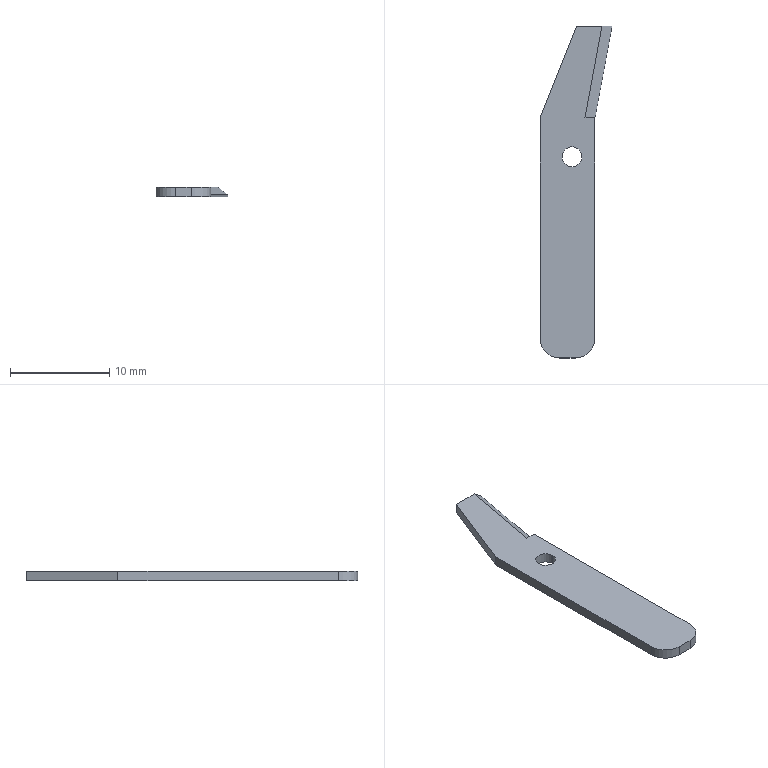Part | SolidWorks | features BaseBody 1, ICE 1 | 1 solid | 14 faces | box 7.242 x 33.391 x 1 mm | volume 166.861 mm3 | plane 10 | cylinder 4 | commonest cylinder face diameters 2 x2 4 x2
STEP:
#1=CARTESIAN_POINT('',(-123.21,229.702,181.));
#2=VERTEX_POINT('',#1);
#3=CARTESIAN_POINT('',(-121.21,229.702,181.));
#4=VERTEX_POINT('',#3);
#5=CARTESIAN_POINT('',(-122.21,229.702,181.));
#6=DIRECTION('',(0.,0.,1.));
#7=DIRECTION('',(0.,-1.,0.));
#8=AXIS2_PLACEMENT_3D('',#5,#6,#7);
#9=CIRCLE('',#8,1.);
#10=EDGE_CURVE('',#2,#4,#9,.T.);
#11=ORIENTED_EDGE('',*,*,#10,.T.);
#12=CARTESIAN_POINT('',(-121.21,229.702,180.));
#13=VERTEX_POINT('',#12);
#14=CARTESIAN_POINT('',(-121.21,229.702,181.));
#15=DIRECTION('',(0.,0.,-1.));
#16=VECTOR('',#15,1000.);
#17=LINE('',#14,#16);
#18=EDGE_CURVE('',#4,#13,#17,.T.);
#19=ORIENTED_EDGE('',*,*,#18,.T.);
#20=CARTESIAN_POINT('',(-123.21,229.702,180.));
#21=VERTEX_POINT('',#20);
#22=CARTESIAN_POINT('',(-122.21,229.702,180.));
#23=DIRECTION('',(0.,0.,1.));
#24=DIRECTION('',(0.,-1.,0.));
#25=AXIS2_PLACEMENT_3D('',#22,#23,#24);
#26=CIRCLE('',#25,1.);
#27=EDGE_CURVE('',#21,#13,#26,.T.);
#28=ORIENTED_EDGE('',*,*,#27,.F.);
#29=CARTESIAN_POINT('',(-123.21,229.702,181.));
#30=DIRECTION('',(0.,0.,-1.));
#31=VECTOR('',#30,1000.);
#32=LINE('',#29,#31);
#33=EDGE_CURVE('',#2,#21,#32,.T.);
#34=ORIENTED_EDGE('',*,*,#33,.F.);
#35=EDGE_LOOP('',(#11,#19,#28,#34));
#36=FACE_OUTER_BOUND('',#35,.T.);
#37=CARTESIAN_POINT('',(-122.21,229.702,181.));
#38=DIRECTION('',(0.,0.,-1.));
#39=DIRECTION('',(-1.,0.,0.));
#40=AXIS2_PLACEMENT_3D('',#37,#38,#39);
#41=CYLINDRICAL_SURFACE('',#40,1.);
#42=ADVANCED_FACE('',(#36),#41,.F.);
#43=CARTESIAN_POINT('',(-125.427,233.602,180.));
#44=VERTEX_POINT('',#43);
#45=CARTESIAN_POINT('',(-125.427,211.461,180.));
#46=VERTEX_POINT('',#45);
#47=CARTESIAN_POINT('',(-125.427,233.602,180.));
#48=DIRECTION('',(0.,-1.,0.));
#49=VECTOR('',#48,1000.);
#50=LINE('',#47,#49);
#51=EDGE_CURVE('',#44,#46,#50,.T.);
#52=ORIENTED_EDGE('',*,*,#51,.T.);
#53=CARTESIAN_POINT('',(-125.427,211.461,181.));
#54=VERTEX_POINT('',#53);
#55=CARTESIAN_POINT('',(-125.427,211.461,180.));
#56=DIRECTION('',(0.,0.,1.));
#57=VECTOR('',#56,1000.);
#58=LINE('',#55,#57);
#59=EDGE_CURVE('',#46,#54,#58,.T.);
#60=ORIENTED_EDGE('',*,*,#59,.T.);
#61=CARTESIAN_POINT('',(-125.427,233.602,181.));
#62=VERTEX_POINT('',#61);
#63=CARTESIAN_POINT('',(-125.427,233.602,181.));
#64=DIRECTION('',(0.,-1.,0.));
#65=VECTOR('',#64,1000.);
#66=LINE('',#63,#65);
#67=EDGE_CURVE('',#62,#54,#66,.T.);
#68=ORIENTED_EDGE('',*,*,#67,.F.);
#69=CARTESIAN_POINT('',(-125.427,233.602,181.));
#70=DIRECTION('',(0.,0.,-1.));
#71=VECTOR('',#70,1000.);
#72=LINE('',#69,#71);
#73=EDGE_CURVE('',#62,#44,#72,.T.);
#74=ORIENTED_EDGE('',*,*,#73,.T.);
#75=EDGE_LOOP('',(#52,#60,#68,#74));
#76=FACE_OUTER_BOUND('',#75,.T.);
#77=CARTESIAN_POINT('',(-125.427,233.602,181.));
#78=DIRECTION('',(1.,0.,0.));
#79=DIRECTION('',(0.,0.,-1.));
#80=AXIS2_PLACEMENT_3D('',#77,#78,#79);
#81=PLANE('',#80);
#82=ADVANCED_FACE('',(#76),#81,.F.);
#83=CARTESIAN_POINT('',(-119.902,233.602,180.2));
#84=VERTEX_POINT('',#83);
#85=CARTESIAN_POINT('',(-119.902,233.602,181.));
#86=VERTEX_POINT('',#85);
#87=CARTESIAN_POINT('',(-119.902,233.602,180.));
#88=DIRECTION('',(0.,0.,1.));
#89=VECTOR('',#88,1000.);
#90=LINE('',#87,#89);
#91=EDGE_CURVE('',#84,#86,#90,.T.);
#92=ORIENTED_EDGE('',*,*,#91,.T.);
#93=CARTESIAN_POINT('',(-119.902,211.461,181.));
#94=VERTEX_POINT('',#93);
#95=CARTESIAN_POINT('',(-119.902,220.3,181.));
#96=DIRECTION('',(0.,1.,0.));
#97=VECTOR('',#96,1000.);
#98=LINE('',#95,#97);
#99=EDGE_CURVE('',#94,#86,#98,.T.);
#100=ORIENTED_EDGE('',*,*,#99,.F.);
#101=CARTESIAN_POINT('',(-119.902,211.461,180.));
#102=VERTEX_POINT('',#101);
#103=CARTESIAN_POINT('',(-119.902,211.461,180.));
#104=DIRECTION('',(0.,0.,1.));
#105=VECTOR('',#104,1000.);
#106=LINE('',#103,#105);
#107=EDGE_CURVE('',#102,#94,#106,.T.);
#108=ORIENTED_EDGE('',*,*,#107,.F.);
#109=CARTESIAN_POINT('',(-119.902,233.602,180.));
#110=VERTEX_POINT('',#109);
#111=CARTESIAN_POINT('',(-119.902,220.3,180.));
#112=DIRECTION('',(0.,1.,0.));
#113=VECTOR('',#112,1000.);
#114=LINE('',#111,#113);
#115=EDGE_CURVE('',#102,#110,#114,.T.);
#116=ORIENTED_EDGE('',*,*,#115,.T.);
#117=CARTESIAN_POINT('',(-119.902,233.602,181.));
#118=DIRECTION('',(0.,0.,-1.));
#119=VECTOR('',#118,1000.);
#120=LINE('',#117,#119);
#121=EDGE_CURVE('',#84,#110,#120,.T.);
#122=ORIENTED_EDGE('',*,*,#121,.F.);
#123=EDGE_LOOP('',(#92,#100,#108,#116,#122));
#124=FACE_OUTER_BOUND('',#123,.T.);
#125=CARTESIAN_POINT('',(-119.902,220.3,181.));
#126=DIRECTION('',(-1.,0.,0.));
#127=DIRECTION('',(0.,0.,1.));
#128=AXIS2_PLACEMENT_3D('',#125,#126,#127);
#129=PLANE('',#128);
#130=ADVANCED_FACE('',(#124),#129,.F.);
#131=CARTESIAN_POINT('',(-118.186,242.853,180.2));
#132=VERTEX_POINT('',#131);
#133=CARTESIAN_POINT('',(-118.186,242.853,180.));
#134=VERTEX_POINT('',#133);
#135=CARTESIAN_POINT('',(-118.186,242.853,181.));
#136=DIRECTION('',(0.,0.,-1.));
#137=VECTOR('',#136,1000.);
#138=LINE('',#135,#137);
#139=EDGE_CURVE('',#132,#134,#138,.T.);
#140=ORIENTED_EDGE('',*,*,#139,.F.);
#141=CARTESIAN_POINT('',(-119.902,233.602,180.2));
#142=DIRECTION('',(-0.1825,-0.9832,0.));
#143=VECTOR('',#142,1000.);
#144=LINE('',#141,#143);
#145=EDGE_CURVE('',#132,#84,#144,.T.);
#146=ORIENTED_EDGE('',*,*,#145,.T.);
#147=ORIENTED_EDGE('',*,*,#121,.T.);
#148=CARTESIAN_POINT('',(-119.902,233.602,180.));
#149=DIRECTION('',(0.1825,0.9832,0.));
#150=VECTOR('',#149,1000.);
#151=LINE('',#148,#150);
#152=EDGE_CURVE('',#110,#134,#151,.T.);
#153=ORIENTED_EDGE('',*,*,#152,.T.);
#154=EDGE_LOOP('',(#140,#146,#147,#153));
#155=FACE_OUTER_BOUND('',#154,.T.);
#156=CARTESIAN_POINT('',(-119.902,233.602,181.));
#157=DIRECTION('',(-0.9832,0.1825,0.));
#158=DIRECTION('',(-0.1825,-0.9832,0.));
#159=AXIS2_PLACEMENT_3D('',#156,#157,#158);
#160=PLANE('',#159);
#161=ADVANCED_FACE('',(#155),#160,.F.);
#162=CARTESIAN_POINT('',(-119.203,242.853,181.));
#163=VERTEX_POINT('',#162);
#164=CARTESIAN_POINT('',(-121.763,242.853,181.));
#165=VERTEX_POINT('',#164);
#166=CARTESIAN_POINT('',(-118.186,242.853,181.));
#167=DIRECTION('',(-1.,0.,0.));
#168=VECTOR('',#167,1000.);
#169=LINE('',#166,#168);
#170=EDGE_CURVE('',#163,#165,#169,.T.);
#171=ORIENTED_EDGE('',*,*,#170,.F.);
#172=CARTESIAN_POINT('',(-120.722,242.853,182.195));
#173=DIRECTION('',(0.786,0.,-0.6182));
#174=VECTOR('',#173,1000.);
#175=LINE('',#172,#174);
#176=EDGE_CURVE('',#163,#132,#175,.T.);
#177=ORIENTED_EDGE('',*,*,#176,.T.);
#178=ORIENTED_EDGE('',*,*,#139,.T.);
#179=CARTESIAN_POINT('',(-121.763,242.853,180.));
#180=VERTEX_POINT('',#179);
#181=CARTESIAN_POINT('',(-118.186,242.853,180.));
#182=DIRECTION('',(-1.,0.,0.));
#183=VECTOR('',#182,1000.);
#184=LINE('',#181,#183);
#185=EDGE_CURVE('',#134,#180,#184,.T.);
#186=ORIENTED_EDGE('',*,*,#185,.T.);
#187=CARTESIAN_POINT('',(-121.763,242.853,181.));
#188=DIRECTION('',(0.,0.,-1.));
#189=VECTOR('',#188,1000.);
#190=LINE('',#187,#189);
#191=EDGE_CURVE('',#165,#180,#190,.T.);
#192=ORIENTED_EDGE('',*,*,#191,.F.);
#193=EDGE_LOOP('',(#171,#177,#178,#186,#192));
#194=FACE_OUTER_BOUND('',#193,.T.);
#195=CARTESIAN_POINT('',(-118.186,242.853,181.));
#196=DIRECTION('',(0.,-1.,0.));
#197=DIRECTION('',(0.,0.,-1.));
#198=AXIS2_PLACEMENT_3D('',#195,#196,#197);
#199=PLANE('',#198);
#200=ADVANCED_FACE('',(#194),#199,.F.);
#201=CARTESIAN_POINT('',(-121.763,242.853,180.));
#202=DIRECTION('',(-0.3683,-0.9297,0.));
#203=VECTOR('',#202,1000.);
#204=LINE('',#201,#203);
#205=EDGE_CURVE('',#180,#44,#204,.T.);
#206=ORIENTED_EDGE('',*,*,#205,.T.);
#207=ORIENTED_EDGE('',*,*,#73,.F.);
#208=CARTESIAN_POINT('',(-121.763,242.853,181.));
#209=DIRECTION('',(-0.3683,-0.9297,0.));
#210=VECTOR('',#209,1000.);
#211=LINE('',#208,#210);
#212=EDGE_CURVE('',#165,#62,#211,.T.);
#213=ORIENTED_EDGE('',*,*,#212,.F.);
#214=ORIENTED_EDGE('',*,*,#191,.T.);
#215=EDGE_LOOP('',(#206,#207,#213,#214));
#216=FACE_OUTER_BOUND('',#215,.T.);
#217=CARTESIAN_POINT('',(-121.763,242.853,181.));
#218=DIRECTION('',(0.9297,-0.3683,0.));
#219=DIRECTION('',(0.3683,0.9297,0.));
#220=AXIS2_PLACEMENT_3D('',#217,#218,#219);
#221=PLANE('',#220);
#222=ADVANCED_FACE('',(#216),#221,.F.);
#223=ORIENTED_EDGE('',*,*,#18,.F.);
#224=CARTESIAN_POINT('',(-122.21,229.702,181.));
#225=DIRECTION('',(0.,0.,1.));
#226=DIRECTION('',(0.,-1.,0.));
#227=AXIS2_PLACEMENT_3D('',#224,#225,#226);
#228=CIRCLE('',#227,1.);
#229=EDGE_CURVE('',#4,#2,#228,.T.);
#230=ORIENTED_EDGE('',*,*,#229,.T.);
#231=ORIENTED_EDGE('',*,*,#33,.T.);
#232=CARTESIAN_POINT('',(-122.21,229.702,180.));
#233=DIRECTION('',(0.,0.,1.));
#234=DIRECTION('',(0.,-1.,0.));
#235=AXIS2_PLACEMENT_3D('',#232,#233,#234);
#236=CIRCLE('',#235,1.);
#237=EDGE_CURVE('',#13,#21,#236,.T.);
#238=ORIENTED_EDGE('',*,*,#237,.F.);
#239=EDGE_LOOP('',(#223,#230,#231,#238));
#240=FACE_OUTER_BOUND('',#239,.T.);
#241=CARTESIAN_POINT('',(-122.21,229.702,181.));
#242=DIRECTION('',(0.,0.,-1.));
#243=DIRECTION('',(-1.,0.,0.));
#244=AXIS2_PLACEMENT_3D('',#241,#242,#243);
#245=CYLINDRICAL_SURFACE('',#244,1.);
#246=ADVANCED_FACE('',(#240),#245,.F.);
#247=ORIENTED_EDGE('',*,*,#67,.T.);
#248=CARTESIAN_POINT('',(-123.427,209.461,181.));
#249=VERTEX_POINT('',#248);
#250=CARTESIAN_POINT('',(-123.427,211.461,181.));
#251=DIRECTION('',(0.,0.,1.));
#252=DIRECTION('',(1.,0.,0.));
#253=AXIS2_PLACEMENT_3D('',#250,#251,#252);
#254=CIRCLE('',#253,2.);
#255=EDGE_CURVE('',#54,#249,#254,.T.);
#256=ORIENTED_EDGE('',*,*,#255,.T.);
#257=CARTESIAN_POINT('',(-121.902,209.461,181.));
#258=VERTEX_POINT('',#257);
#259=CARTESIAN_POINT('',(-123.427,209.461,181.));
#260=DIRECTION('',(1.,0.,0.));
#261=VECTOR('',#260,1000.);
#262=LINE('',#259,#261);
#263=EDGE_CURVE('',#249,#258,#262,.T.);
#264=ORIENTED_EDGE('',*,*,#263,.T.);
#265=CARTESIAN_POINT('',(-121.902,211.461,181.));
#266=DIRECTION('',(0.,0.,1.));
#267=DIRECTION('',(-1.,0.,0.));
#268=AXIS2_PLACEMENT_3D('',#265,#266,#267);
#269=CIRCLE('',#268,2.);
#270=EDGE_CURVE('',#258,#94,#269,.T.);
#271=ORIENTED_EDGE('',*,*,#270,.T.);
#272=ORIENTED_EDGE('',*,*,#99,.T.);
#273=CARTESIAN_POINT('',(-120.902,233.694,181.));
#274=VERTEX_POINT('',#273);
#275=CARTESIAN_POINT('',(-119.902,233.602,181.));
#276=DIRECTION('',(-0.9958,0.09162,0.));
#277=VECTOR('',#276,1000.);
#278=LINE('',#275,#277);
#279=EDGE_CURVE('',#86,#274,#278,.T.);
#280=ORIENTED_EDGE('',*,*,#279,.T.);
#281=CARTESIAN_POINT('',(-119.169,243.035,181.));
#282=DIRECTION('',(0.1825,0.9832,0.));
#283=VECTOR('',#282,1000.);
#284=LINE('',#281,#283);
#285=EDGE_CURVE('',#274,#163,#284,.T.);
#286=ORIENTED_EDGE('',*,*,#285,.T.);
#287=ORIENTED_EDGE('',*,*,#170,.T.);
#288=ORIENTED_EDGE('',*,*,#212,.T.);
#289=EDGE_LOOP('',(#247,#256,#264,#271,#272,#280,#286,#287,#288));
#290=FACE_OUTER_BOUND('',#289,.T.);
#291=ORIENTED_EDGE('',*,*,#10,.F.);
#292=ORIENTED_EDGE('',*,*,#229,.F.);
#293=EDGE_LOOP('',(#291,#292));
#294=FACE_BOUND('',#293,.T.);
#295=CARTESIAN_POINT('',(-122.21,229.702,181.));
#296=DIRECTION('',(0.,0.,1.));
#297=DIRECTION('',(1.,0.,0.));
#298=AXIS2_PLACEMENT_3D('',#295,#296,#297);
#299=PLANE('',#298);
#300=ADVANCED_FACE('',(#290,#294),#299,.T.);
#301=ORIENTED_EDGE('',*,*,#152,.F.);
#302=ORIENTED_EDGE('',*,*,#115,.F.);
#303=CARTESIAN_POINT('',(-121.902,209.461,180.));
#304=VERTEX_POINT('',#303);
#305=CARTESIAN_POINT('',(-121.902,211.461,180.));
#306=DIRECTION('',(0.,0.,1.));
#307=DIRECTION('',(-1.,0.,0.));
#308=AXIS2_PLACEMENT_3D('',#305,#306,#307);
#309=CIRCLE('',#308,2.);
#310=EDGE_CURVE('',#304,#102,#309,.T.);
#311=ORIENTED_EDGE('',*,*,#310,.F.);
#312=CARTESIAN_POINT('',(-123.427,209.461,180.));
#313=VERTEX_POINT('',#312);
#314=CARTESIAN_POINT('',(-123.427,209.461,180.));
#315=DIRECTION('',(1.,0.,0.));
#316=VECTOR('',#315,1000.);
#317=LINE('',#314,#316);
#318=EDGE_CURVE('',#313,#304,#317,.T.);
#319=ORIENTED_EDGE('',*,*,#318,.F.);
#320=CARTESIAN_POINT('',(-123.427,211.461,180.));
#321=DIRECTION('',(0.,0.,1.));
#322=DIRECTION('',(1.,0.,0.));
#323=AXIS2_PLACEMENT_3D('',#320,#321,#322);
#324=CIRCLE('',#323,2.);
#325=EDGE_CURVE('',#46,#313,#324,.T.);
#326=ORIENTED_EDGE('',*,*,#325,.F.);
#327=ORIENTED_EDGE('',*,*,#51,.F.);
#328=ORIENTED_EDGE('',*,*,#205,.F.);
#329=ORIENTED_EDGE('',*,*,#185,.F.);
#330=EDGE_LOOP('',(#301,#302,#311,#319,#326,#327,#328,#329));
#331=FACE_OUTER_BOUND('',#330,.T.);
#332=ORIENTED_EDGE('',*,*,#27,.T.);
#333=ORIENTED_EDGE('',*,*,#237,.T.);
#334=EDGE_LOOP('',(#332,#333));
#335=FACE_BOUND('',#334,.T.);
#336=CARTESIAN_POINT('',(-122.21,229.702,180.));
#337=DIRECTION('',(0.,0.,1.));
#338=DIRECTION('',(1.,0.,0.));
#339=AXIS2_PLACEMENT_3D('',#336,#337,#338);
#340=PLANE('',#339);
#341=ADVANCED_FACE('',(#331,#335),#340,.F.);
#342=ORIENTED_EDGE('',*,*,#176,.F.);
#343=ORIENTED_EDGE('',*,*,#285,.F.);
#344=CARTESIAN_POINT('',(-120.68,233.673,180.822));
#345=DIRECTION('',(-0.7789,0.07166,0.6231));
#346=VECTOR('',#345,1000.);
#347=LINE('',#344,#346);
#348=EDGE_CURVE('',#84,#274,#347,.T.);
#349=ORIENTED_EDGE('',*,*,#348,.F.);
#350=ORIENTED_EDGE('',*,*,#145,.F.);
#351=EDGE_LOOP('',(#342,#343,#349,#350));
#352=FACE_OUTER_BOUND('',#351,.T.);
#353=CARTESIAN_POINT('',(-121.662,229.6,181.));
#354=DIRECTION('',(0.6142,-0.114,0.7809));
#355=DIRECTION('',(-0.1825,-0.9832,0.));
#356=AXIS2_PLACEMENT_3D('',#353,#354,#355);
#357=PLANE('',#356);
#358=ADVANCED_FACE('',(#352),#357,.T.);
#359=ORIENTED_EDGE('',*,*,#91,.F.);
#360=ORIENTED_EDGE('',*,*,#348,.T.);
#361=ORIENTED_EDGE('',*,*,#279,.F.);
#362=EDGE_LOOP('',(#359,#360,#361));
#363=FACE_OUTER_BOUND('',#362,.T.);
#364=CARTESIAN_POINT('',(-119.902,233.602,180.));
#365=DIRECTION('',(0.09162,0.9958,0.));
#366=DIRECTION('',(-0.9958,0.09162,0.));
#367=AXIS2_PLACEMENT_3D('',#364,#365,#366);
#368=PLANE('',#367);
#369=ADVANCED_FACE('',(#363),#368,.T.);
#370=ORIENTED_EDGE('',*,*,#270,.F.);
#371=CARTESIAN_POINT('',(-121.902,209.461,180.));
#372=DIRECTION('',(0.,0.,1.));
#373=VECTOR('',#372,1000.);
#374=LINE('',#371,#373);
#375=EDGE_CURVE('',#304,#258,#374,.T.);
#376=ORIENTED_EDGE('',*,*,#375,.F.);
#377=ORIENTED_EDGE('',*,*,#310,.T.);
#378=ORIENTED_EDGE('',*,*,#107,.T.);
#379=EDGE_LOOP('',(#370,#376,#377,#378));
#380=FACE_OUTER_BOUND('',#379,.T.);
#381=CARTESIAN_POINT('',(-121.902,211.461,180.));
#382=DIRECTION('',(0.,0.,1.));
#383=DIRECTION('',(1.,0.,0.));
#384=AXIS2_PLACEMENT_3D('',#381,#382,#383);
#385=CYLINDRICAL_SURFACE('',#384,2.);
#386=ADVANCED_FACE('',(#380),#385,.T.);
#387=ORIENTED_EDGE('',*,*,#263,.F.);
#388=CARTESIAN_POINT('',(-123.427,209.461,180.));
#389=DIRECTION('',(0.,0.,1.));
#390=VECTOR('',#389,1000.);
#391=LINE('',#388,#390);
#392=EDGE_CURVE('',#313,#249,#391,.T.);
#393=ORIENTED_EDGE('',*,*,#392,.F.);
#394=ORIENTED_EDGE('',*,*,#318,.T.);
#395=ORIENTED_EDGE('',*,*,#375,.T.);
#396=EDGE_LOOP('',(#387,#393,#394,#395));
#397=FACE_OUTER_BOUND('',#396,.T.);
#398=CARTESIAN_POINT('',(-123.427,209.461,180.));
#399=DIRECTION('',(0.,-1.,0.));
#400=DIRECTION('',(0.,0.,-1.));
#401=AXIS2_PLACEMENT_3D('',#398,#399,#400);
#402=PLANE('',#401);
#403=ADVANCED_FACE('',(#397),#402,.T.);
#404=ORIENTED_EDGE('',*,*,#255,.F.);
#405=ORIENTED_EDGE('',*,*,#59,.F.);
#406=ORIENTED_EDGE('',*,*,#325,.T.);
#407=ORIENTED_EDGE('',*,*,#392,.T.);
#408=EDGE_LOOP('',(#404,#405,#406,#407));
#409=FACE_OUTER_BOUND('',#408,.T.);
#410=CARTESIAN_POINT('',(-123.427,211.461,180.));
#411=DIRECTION('',(0.,0.,1.));
#412=DIRECTION('',(1.,0.,0.));
#413=AXIS2_PLACEMENT_3D('',#410,#411,#412);
#414=CYLINDRICAL_SURFACE('',#413,2.);
#415=ADVANCED_FACE('',(#409),#414,.T.);
#416=CLOSED_SHELL('',(#42,#82,#130,#161,#200,#222,#246,#300,#341,#358,#369,#386,#403,#415));
#417=MANIFOLD_SOLID_BREP('',#416);
#418=CARTESIAN_POINT('',(0.,0.,0.));
#419=DIRECTION('',(0.,0.,1.));
#420=DIRECTION('',(1.,0.,0.));
#421=AXIS2_PLACEMENT_3D('',#418,#419,#420);
#422=(LENGTH_UNIT()NAMED_UNIT(*)SI_UNIT(.MILLI.,.METRE.));
#423=UNCERTAINTY_MEASURE_WITH_UNIT(LENGTH_MEASURE(0.00001),#422,'','');
#424=(NAMED_UNIT(*)PLANE_ANGLE_UNIT()SI_UNIT($,.RADIAN.));
#425=(NAMED_UNIT(*)SI_UNIT($,.STERADIAN.)SOLID_ANGLE_UNIT());
#426=(GEOMETRIC_REPRESENTATION_CONTEXT(3)GLOBAL_UNCERTAINTY_ASSIGNED_CONTEXT((#423))GLOBAL_UNIT_ASSIGNED_CONTEXT((#422,#424,#425))REPRESENTATION_CONTEXT('',''));
#427=ADVANCED_BREP_SHAPE_REPRESENTATION('',(#417,#421),#426);